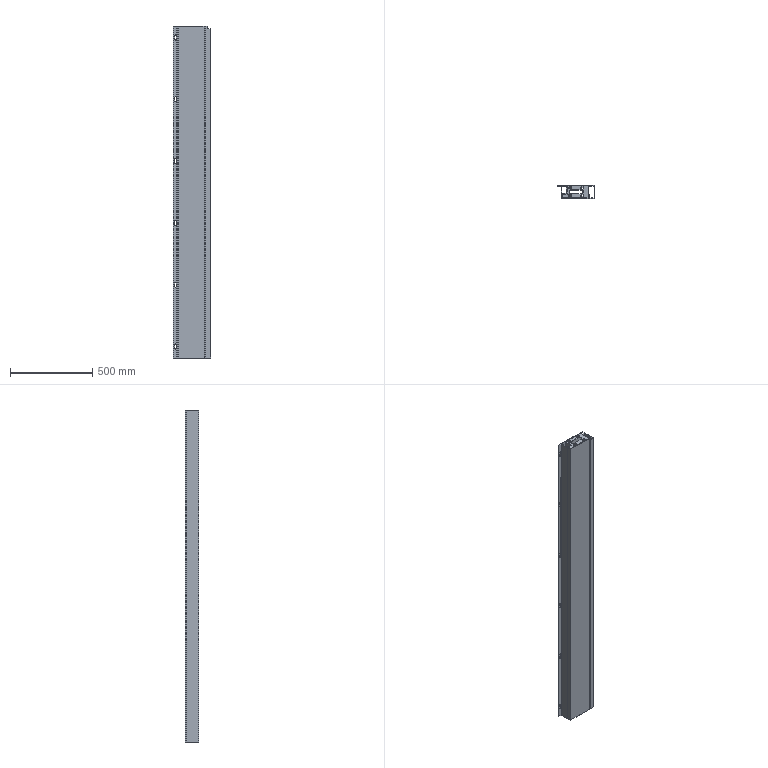Part | 5 solids | 154 faces | box 225 x 80 x 2016 mm | volume 3151797 mm3 | plane 88 | cylinder 66 | commonest cylinder face diameters 10 x24 9 x18 2 x9 6 x8 25 x6 8 x1